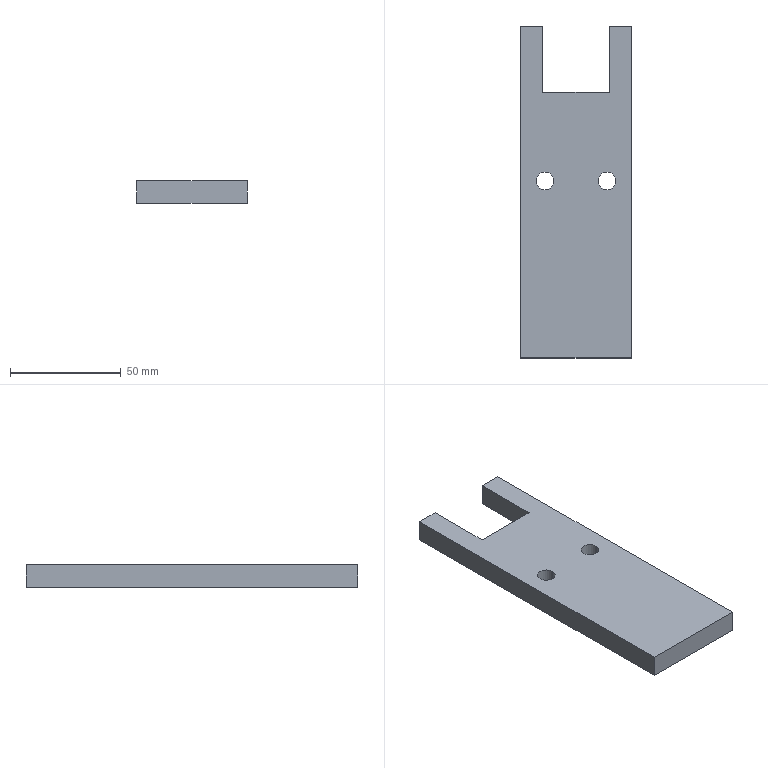Part | SolidWorks | features ICE 2, Extrusion 1 | 1 solid | 14 faces | box 50 x 150 x 10 mm | volume 64995 mm3 | plane 10 | cylinder 4 | commonest cylinder face diameters 8 x4
STEP:
#1=CARTESIAN_POINT('',(-18.,5.,0.));
#2=VERTEX_POINT('',#1);
#3=CARTESIAN_POINT('',(-10.,5.,0.));
#4=VERTEX_POINT('',#3);
#5=CARTESIAN_POINT('',(-14.,5.,0.));
#6=DIRECTION('',(0.,0.,1.));
#7=DIRECTION('',(1.,0.,0.));
#8=AXIS2_PLACEMENT_3D('',#5,#6,#7);
#9=CIRCLE('',#8,4.);
#10=EDGE_CURVE('',#2,#4,#9,.T.);
#11=ORIENTED_EDGE('',*,*,#10,.F.);
#12=CARTESIAN_POINT('',(-18.,5.,10.));
#13=VERTEX_POINT('',#12);
#14=CARTESIAN_POINT('',(-18.,5.,0.));
#15=DIRECTION('',(0.,0.,1.));
#16=VECTOR('',#15,1000.);
#17=LINE('',#14,#16);
#18=EDGE_CURVE('',#2,#13,#17,.T.);
#19=ORIENTED_EDGE('',*,*,#18,.T.);
#20=CARTESIAN_POINT('',(-10.,5.,10.));
#21=VERTEX_POINT('',#20);
#22=CARTESIAN_POINT('',(-14.,5.,10.));
#23=DIRECTION('',(0.,0.,1.));
#24=DIRECTION('',(1.,0.,0.));
#25=AXIS2_PLACEMENT_3D('',#22,#23,#24);
#26=CIRCLE('',#25,4.);
#27=EDGE_CURVE('',#13,#21,#26,.T.);
#28=ORIENTED_EDGE('',*,*,#27,.T.);
#29=CARTESIAN_POINT('',(-10.,5.,0.));
#30=DIRECTION('',(0.,0.,1.));
#31=VECTOR('',#30,1000.);
#32=LINE('',#29,#31);
#33=EDGE_CURVE('',#4,#21,#32,.T.);
#34=ORIENTED_EDGE('',*,*,#33,.F.);
#35=EDGE_LOOP('',(#11,#19,#28,#34));
#36=FACE_OUTER_BOUND('',#35,.T.);
#37=CARTESIAN_POINT('',(-14.,5.,0.));
#38=DIRECTION('',(0.,0.,1.));
#39=DIRECTION('',(1.,0.,0.));
#40=AXIS2_PLACEMENT_3D('',#37,#38,#39);
#41=CYLINDRICAL_SURFACE('',#40,4.);
#42=ADVANCED_FACE('',(#36),#41,.F.);
#43=CARTESIAN_POINT('',(10.,5.,0.));
#44=VERTEX_POINT('',#43);
#45=CARTESIAN_POINT('',(18.,5.,0.));
#46=VERTEX_POINT('',#45);
#47=CARTESIAN_POINT('',(14.,5.,0.));
#48=DIRECTION('',(0.,0.,1.));
#49=DIRECTION('',(-1.,0.,0.));
#50=AXIS2_PLACEMENT_3D('',#47,#48,#49);
#51=CIRCLE('',#50,4.);
#52=EDGE_CURVE('',#44,#46,#51,.T.);
#53=ORIENTED_EDGE('',*,*,#52,.F.);
#54=CARTESIAN_POINT('',(10.,5.,10.));
#55=VERTEX_POINT('',#54);
#56=CARTESIAN_POINT('',(10.,5.,0.));
#57=DIRECTION('',(0.,0.,1.));
#58=VECTOR('',#57,1000.);
#59=LINE('',#56,#58);
#60=EDGE_CURVE('',#44,#55,#59,.T.);
#61=ORIENTED_EDGE('',*,*,#60,.T.);
#62=CARTESIAN_POINT('',(18.,5.,10.));
#63=VERTEX_POINT('',#62);
#64=CARTESIAN_POINT('',(14.,5.,10.));
#65=DIRECTION('',(0.,0.,1.));
#66=DIRECTION('',(-1.,0.,0.));
#67=AXIS2_PLACEMENT_3D('',#64,#65,#66);
#68=CIRCLE('',#67,4.);
#69=EDGE_CURVE('',#55,#63,#68,.T.);
#70=ORIENTED_EDGE('',*,*,#69,.T.);
#71=CARTESIAN_POINT('',(18.,5.,0.));
#72=DIRECTION('',(0.,0.,1.));
#73=VECTOR('',#72,1000.);
#74=LINE('',#71,#73);
#75=EDGE_CURVE('',#46,#63,#74,.T.);
#76=ORIENTED_EDGE('',*,*,#75,.F.);
#77=EDGE_LOOP('',(#53,#61,#70,#76));
#78=FACE_OUTER_BOUND('',#77,.T.);
#79=CARTESIAN_POINT('',(14.,5.,0.));
#80=DIRECTION('',(0.,0.,1.));
#81=DIRECTION('',(1.,0.,0.));
#82=AXIS2_PLACEMENT_3D('',#79,#80,#81);
#83=CYLINDRICAL_SURFACE('',#82,4.);
#84=ADVANCED_FACE('',(#78),#83,.F.);
#85=CARTESIAN_POINT('',(-15.,75.,10.));
#86=VERTEX_POINT('',#85);
#87=CARTESIAN_POINT('',(-25.,75.,10.));
#88=VERTEX_POINT('',#87);
#89=CARTESIAN_POINT('',(-25.,75.,10.));
#90=DIRECTION('',(-1.,0.,0.));
#91=VECTOR('',#90,1000.);
#92=LINE('',#89,#91);
#93=EDGE_CURVE('',#86,#88,#92,.T.);
#94=ORIENTED_EDGE('',*,*,#93,.F.);
#95=CARTESIAN_POINT('',(-15.,75.,0.));
#96=VERTEX_POINT('',#95);
#97=CARTESIAN_POINT('',(-15.,75.,0.));
#98=DIRECTION('',(0.,0.,1.));
#99=VECTOR('',#98,1000.);
#100=LINE('',#97,#99);
#101=EDGE_CURVE('',#96,#86,#100,.T.);
#102=ORIENTED_EDGE('',*,*,#101,.F.);
#103=CARTESIAN_POINT('',(-25.,75.,0.));
#104=VERTEX_POINT('',#103);
#105=CARTESIAN_POINT('',(-25.,75.,0.));
#106=DIRECTION('',(-1.,0.,0.));
#107=VECTOR('',#106,1000.);
#108=LINE('',#105,#107);
#109=EDGE_CURVE('',#96,#104,#108,.T.);
#110=ORIENTED_EDGE('',*,*,#109,.T.);
#111=CARTESIAN_POINT('',(-25.,75.,10.));
#112=DIRECTION('',(0.,0.,-1.));
#113=VECTOR('',#112,1000.);
#114=LINE('',#111,#113);
#115=EDGE_CURVE('',#88,#104,#114,.T.);
#116=ORIENTED_EDGE('',*,*,#115,.F.);
#117=EDGE_LOOP('',(#94,#102,#110,#116));
#118=FACE_OUTER_BOUND('',#117,.T.);
#119=CARTESIAN_POINT('',(-25.,75.,10.));
#120=DIRECTION('',(0.,-1.,0.));
#121=DIRECTION('',(0.,0.,-1.));
#122=AXIS2_PLACEMENT_3D('',#119,#120,#121);
#123=PLANE('',#122);
#124=ADVANCED_FACE('',(#118),#123,.F.);
#125=CARTESIAN_POINT('',(25.,-75.,0.));
#126=VERTEX_POINT('',#125);
#127=CARTESIAN_POINT('',(25.,75.,0.));
#128=VERTEX_POINT('',#127);
#129=CARTESIAN_POINT('',(25.,-75.,0.));
#130=DIRECTION('',(0.,1.,0.));
#131=VECTOR('',#130,1000.);
#132=LINE('',#129,#131);
#133=EDGE_CURVE('',#126,#128,#132,.T.);
#134=ORIENTED_EDGE('',*,*,#133,.T.);
#135=CARTESIAN_POINT('',(25.,75.,10.));
#136=VERTEX_POINT('',#135);
#137=CARTESIAN_POINT('',(25.,75.,10.));
#138=DIRECTION('',(0.,0.,-1.));
#139=VECTOR('',#138,1000.);
#140=LINE('',#137,#139);
#141=EDGE_CURVE('',#136,#128,#140,.T.);
#142=ORIENTED_EDGE('',*,*,#141,.F.);
#143=CARTESIAN_POINT('',(25.,-75.,10.));
#144=VERTEX_POINT('',#143);
#145=CARTESIAN_POINT('',(25.,-75.,10.));
#146=DIRECTION('',(0.,1.,0.));
#147=VECTOR('',#146,1000.);
#148=LINE('',#145,#147);
#149=EDGE_CURVE('',#144,#136,#148,.T.);
#150=ORIENTED_EDGE('',*,*,#149,.F.);
#151=CARTESIAN_POINT('',(25.,-75.,10.));
#152=DIRECTION('',(0.,0.,-1.));
#153=VECTOR('',#152,1000.);
#154=LINE('',#151,#153);
#155=EDGE_CURVE('',#144,#126,#154,.T.);
#156=ORIENTED_EDGE('',*,*,#155,.T.);
#157=EDGE_LOOP('',(#134,#142,#150,#156));
#158=FACE_OUTER_BOUND('',#157,.T.);
#159=CARTESIAN_POINT('',(25.,-75.,10.));
#160=DIRECTION('',(-1.,0.,0.));
#161=DIRECTION('',(0.,0.,1.));
#162=AXIS2_PLACEMENT_3D('',#159,#160,#161);
#163=PLANE('',#162);
#164=ADVANCED_FACE('',(#158),#163,.F.);
#165=CARTESIAN_POINT('',(15.,75.,0.));
#166=VERTEX_POINT('',#165);
#167=CARTESIAN_POINT('',(-25.,75.,0.));
#168=DIRECTION('',(-1.,0.,0.));
#169=VECTOR('',#168,1000.);
#170=LINE('',#167,#169);
#171=EDGE_CURVE('',#128,#166,#170,.T.);
#172=ORIENTED_EDGE('',*,*,#171,.T.);
#173=CARTESIAN_POINT('',(15.,75.,10.));
#174=VERTEX_POINT('',#173);
#175=CARTESIAN_POINT('',(15.,75.,0.));
#176=DIRECTION('',(0.,0.,1.));
#177=VECTOR('',#176,1000.);
#178=LINE('',#175,#177);
#179=EDGE_CURVE('',#166,#174,#178,.T.);
#180=ORIENTED_EDGE('',*,*,#179,.T.);
#181=CARTESIAN_POINT('',(-25.,75.,10.));
#182=DIRECTION('',(-1.,0.,0.));
#183=VECTOR('',#182,1000.);
#184=LINE('',#181,#183);
#185=EDGE_CURVE('',#136,#174,#184,.T.);
#186=ORIENTED_EDGE('',*,*,#185,.F.);
#187=ORIENTED_EDGE('',*,*,#141,.T.);
#188=EDGE_LOOP('',(#172,#180,#186,#187));
#189=FACE_OUTER_BOUND('',#188,.T.);
#190=CARTESIAN_POINT('',(-25.,75.,10.));
#191=DIRECTION('',(0.,-1.,0.));
#192=DIRECTION('',(0.,0.,-1.));
#193=AXIS2_PLACEMENT_3D('',#190,#191,#192);
#194=PLANE('',#193);
#195=ADVANCED_FACE('',(#189),#194,.F.);
#196=CARTESIAN_POINT('',(-25.,-75.,0.));
#197=VERTEX_POINT('',#196);
#198=CARTESIAN_POINT('',(-25.,-75.,0.));
#199=DIRECTION('',(0.,-1.,0.));
#200=VECTOR('',#199,1000.);
#201=LINE('',#198,#200);
#202=EDGE_CURVE('',#104,#197,#201,.T.);
#203=ORIENTED_EDGE('',*,*,#202,.T.);
#204=CARTESIAN_POINT('',(-25.,-75.,10.));
#205=VERTEX_POINT('',#204);
#206=CARTESIAN_POINT('',(-25.,-75.,10.));
#207=DIRECTION('',(0.,0.,-1.));
#208=VECTOR('',#207,1000.);
#209=LINE('',#206,#208);
#210=EDGE_CURVE('',#205,#197,#209,.T.);
#211=ORIENTED_EDGE('',*,*,#210,.F.);
#212=CARTESIAN_POINT('',(-25.,-75.,10.));
#213=DIRECTION('',(0.,-1.,0.));
#214=VECTOR('',#213,1000.);
#215=LINE('',#212,#214);
#216=EDGE_CURVE('',#88,#205,#215,.T.);
#217=ORIENTED_EDGE('',*,*,#216,.F.);
#218=ORIENTED_EDGE('',*,*,#115,.T.);
#219=EDGE_LOOP('',(#203,#211,#217,#218));
#220=FACE_OUTER_BOUND('',#219,.T.);
#221=CARTESIAN_POINT('',(-25.,-75.,10.));
#222=DIRECTION('',(1.,0.,0.));
#223=DIRECTION('',(0.,0.,-1.));
#224=AXIS2_PLACEMENT_3D('',#221,#222,#223);
#225=PLANE('',#224);
#226=ADVANCED_FACE('',(#220),#225,.F.);
#227=CARTESIAN_POINT('',(-25.,-75.,0.));
#228=DIRECTION('',(1.,0.,0.));
#229=VECTOR('',#228,1000.);
#230=LINE('',#227,#229);
#231=EDGE_CURVE('',#197,#126,#230,.T.);
#232=ORIENTED_EDGE('',*,*,#231,.T.);
#233=ORIENTED_EDGE('',*,*,#155,.F.);
#234=CARTESIAN_POINT('',(-25.,-75.,10.));
#235=DIRECTION('',(1.,0.,0.));
#236=VECTOR('',#235,1000.);
#237=LINE('',#234,#236);
#238=EDGE_CURVE('',#205,#144,#237,.T.);
#239=ORIENTED_EDGE('',*,*,#238,.F.);
#240=ORIENTED_EDGE('',*,*,#210,.T.);
#241=EDGE_LOOP('',(#232,#233,#239,#240));
#242=FACE_OUTER_BOUND('',#241,.T.);
#243=CARTESIAN_POINT('',(-25.,-75.,10.));
#244=DIRECTION('',(0.,1.,0.));
#245=DIRECTION('',(0.,0.,1.));
#246=AXIS2_PLACEMENT_3D('',#243,#244,#245);
#247=PLANE('',#246);
#248=ADVANCED_FACE('',(#242),#247,.F.);
#249=CARTESIAN_POINT('',(-14.,5.,10.));
#250=DIRECTION('',(0.,0.,1.));
#251=DIRECTION('',(1.,0.,0.));
#252=AXIS2_PLACEMENT_3D('',#249,#250,#251);
#253=CIRCLE('',#252,4.);
#254=EDGE_CURVE('',#21,#13,#253,.T.);
#255=ORIENTED_EDGE('',*,*,#254,.F.);
#256=ORIENTED_EDGE('',*,*,#27,.F.);
#257=EDGE_LOOP('',(#255,#256));
#258=FACE_BOUND('',#257,.T.);
#259=CARTESIAN_POINT('',(14.,5.,10.));
#260=DIRECTION('',(0.,0.,1.));
#261=DIRECTION('',(-1.,0.,0.));
#262=AXIS2_PLACEMENT_3D('',#259,#260,#261);
#263=CIRCLE('',#262,4.);
#264=EDGE_CURVE('',#63,#55,#263,.T.);
#265=ORIENTED_EDGE('',*,*,#264,.F.);
#266=ORIENTED_EDGE('',*,*,#69,.F.);
#267=EDGE_LOOP('',(#265,#266));
#268=FACE_BOUND('',#267,.T.);
#269=CARTESIAN_POINT('',(-15.,45.,10.));
#270=VERTEX_POINT('',#269);
#271=CARTESIAN_POINT('',(15.,45.,10.));
#272=VERTEX_POINT('',#271);
#273=CARTESIAN_POINT('',(-15.,45.,10.));
#274=DIRECTION('',(1.,0.,0.));
#275=VECTOR('',#274,1000.);
#276=LINE('',#273,#275);
#277=EDGE_CURVE('',#270,#272,#276,.T.);
#278=ORIENTED_EDGE('',*,*,#277,.F.);
#279=CARTESIAN_POINT('',(-15.,75.,10.));
#280=DIRECTION('',(0.,-1.,0.));
#281=VECTOR('',#280,1000.);
#282=LINE('',#279,#281);
#283=EDGE_CURVE('',#86,#270,#282,.T.);
#284=ORIENTED_EDGE('',*,*,#283,.F.);
#285=ORIENTED_EDGE('',*,*,#93,.T.);
#286=ORIENTED_EDGE('',*,*,#216,.T.);
#287=ORIENTED_EDGE('',*,*,#238,.T.);
#288=ORIENTED_EDGE('',*,*,#149,.T.);
#289=ORIENTED_EDGE('',*,*,#185,.T.);
#290=CARTESIAN_POINT('',(15.,75.,10.));
#291=DIRECTION('',(0.,1.,0.));
#292=VECTOR('',#291,1000.);
#293=LINE('',#290,#292);
#294=EDGE_CURVE('',#272,#174,#293,.T.);
#295=ORIENTED_EDGE('',*,*,#294,.F.);
#296=EDGE_LOOP('',(#278,#284,#285,#286,#287,#288,#289,#295));
#297=FACE_OUTER_BOUND('',#296,.T.);
#298=CARTESIAN_POINT('',(0.,0.,10.));
#299=DIRECTION('',(0.,0.,-1.));
#300=DIRECTION('',(-1.,0.,0.));
#301=AXIS2_PLACEMENT_3D('',#298,#299,#300);
#302=PLANE('',#301);
#303=ADVANCED_FACE('',(#258,#268,#297),#302,.F.);
#304=CARTESIAN_POINT('',(-14.,5.,0.));
#305=DIRECTION('',(0.,0.,1.));
#306=DIRECTION('',(1.,0.,0.));
#307=AXIS2_PLACEMENT_3D('',#304,#305,#306);
#308=CIRCLE('',#307,4.);
#309=EDGE_CURVE('',#4,#2,#308,.T.);
#310=ORIENTED_EDGE('',*,*,#309,.T.);
#311=ORIENTED_EDGE('',*,*,#10,.T.);
#312=EDGE_LOOP('',(#310,#311));
#313=FACE_BOUND('',#312,.T.);
#314=CARTESIAN_POINT('',(14.,5.,0.));
#315=DIRECTION('',(0.,0.,1.));
#316=DIRECTION('',(-1.,0.,0.));
#317=AXIS2_PLACEMENT_3D('',#314,#315,#316);
#318=CIRCLE('',#317,4.);
#319=EDGE_CURVE('',#46,#44,#318,.T.);
#320=ORIENTED_EDGE('',*,*,#319,.T.);
#321=ORIENTED_EDGE('',*,*,#52,.T.);
#322=EDGE_LOOP('',(#320,#321));
#323=FACE_BOUND('',#322,.T.);
#324=CARTESIAN_POINT('',(-15.,45.,0.));
#325=VERTEX_POINT('',#324);
#326=CARTESIAN_POINT('',(-15.,75.,0.));
#327=DIRECTION('',(0.,-1.,0.));
#328=VECTOR('',#327,1000.);
#329=LINE('',#326,#328);
#330=EDGE_CURVE('',#96,#325,#329,.T.);
#331=ORIENTED_EDGE('',*,*,#330,.T.);
#332=CARTESIAN_POINT('',(15.,45.,0.));
#333=VERTEX_POINT('',#332);
#334=CARTESIAN_POINT('',(-15.,45.,0.));
#335=DIRECTION('',(1.,0.,0.));
#336=VECTOR('',#335,1000.);
#337=LINE('',#334,#336);
#338=EDGE_CURVE('',#325,#333,#337,.T.);
#339=ORIENTED_EDGE('',*,*,#338,.T.);
#340=CARTESIAN_POINT('',(15.,75.,0.));
#341=DIRECTION('',(0.,1.,0.));
#342=VECTOR('',#341,1000.);
#343=LINE('',#340,#342);
#344=EDGE_CURVE('',#333,#166,#343,.T.);
#345=ORIENTED_EDGE('',*,*,#344,.T.);
#346=ORIENTED_EDGE('',*,*,#171,.F.);
#347=ORIENTED_EDGE('',*,*,#133,.F.);
#348=ORIENTED_EDGE('',*,*,#231,.F.);
#349=ORIENTED_EDGE('',*,*,#202,.F.);
#350=ORIENTED_EDGE('',*,*,#109,.F.);
#351=EDGE_LOOP('',(#331,#339,#345,#346,#347,#348,#349,#350));
#352=FACE_OUTER_BOUND('',#351,.T.);
#353=CARTESIAN_POINT('',(0.,0.,0.));
#354=DIRECTION('',(0.,0.,-1.));
#355=DIRECTION('',(-1.,0.,0.));
#356=AXIS2_PLACEMENT_3D('',#353,#354,#355);
#357=PLANE('',#356);
#358=ADVANCED_FACE('',(#313,#323,#352),#357,.T.);
#359=ORIENTED_EDGE('',*,*,#283,.T.);
#360=CARTESIAN_POINT('',(-15.,45.,0.));
#361=DIRECTION('',(0.,0.,1.));
#362=VECTOR('',#361,1000.);
#363=LINE('',#360,#362);
#364=EDGE_CURVE('',#325,#270,#363,.T.);
#365=ORIENTED_EDGE('',*,*,#364,.F.);
#366=ORIENTED_EDGE('',*,*,#330,.F.);
#367=ORIENTED_EDGE('',*,*,#101,.T.);
#368=EDGE_LOOP('',(#359,#365,#366,#367));
#369=FACE_OUTER_BOUND('',#368,.T.);
#370=CARTESIAN_POINT('',(-15.,75.,0.));
#371=DIRECTION('',(-1.,0.,0.));
#372=DIRECTION('',(0.,-1.,0.));
#373=AXIS2_PLACEMENT_3D('',#370,#371,#372);
#374=PLANE('',#373);
#375=ADVANCED_FACE('',(#369),#374,.F.);
#376=ORIENTED_EDGE('',*,*,#294,.T.);
#377=ORIENTED_EDGE('',*,*,#179,.F.);
#378=ORIENTED_EDGE('',*,*,#344,.F.);
#379=CARTESIAN_POINT('',(15.,45.,0.));
#380=DIRECTION('',(0.,0.,1.));
#381=VECTOR('',#380,1000.);
#382=LINE('',#379,#381);
#383=EDGE_CURVE('',#333,#272,#382,.T.);
#384=ORIENTED_EDGE('',*,*,#383,.T.);
#385=EDGE_LOOP('',(#376,#377,#378,#384));
#386=FACE_OUTER_BOUND('',#385,.T.);
#387=CARTESIAN_POINT('',(15.,75.,0.));
#388=DIRECTION('',(1.,0.,0.));
#389=DIRECTION('',(0.,1.,0.));
#390=AXIS2_PLACEMENT_3D('',#387,#388,#389);
#391=PLANE('',#390);
#392=ADVANCED_FACE('',(#386),#391,.F.);
#393=ORIENTED_EDGE('',*,*,#277,.T.);
#394=ORIENTED_EDGE('',*,*,#383,.F.);
#395=ORIENTED_EDGE('',*,*,#338,.F.);
#396=ORIENTED_EDGE('',*,*,#364,.T.);
#397=EDGE_LOOP('',(#393,#394,#395,#396));
#398=FACE_OUTER_BOUND('',#397,.T.);
#399=CARTESIAN_POINT('',(-15.,45.,0.));
#400=DIRECTION('',(0.,-1.,0.));
#401=DIRECTION('',(0.,0.,-1.));
#402=AXIS2_PLACEMENT_3D('',#399,#400,#401);
#403=PLANE('',#402);
#404=ADVANCED_FACE('',(#398),#403,.F.);
#405=ORIENTED_EDGE('',*,*,#60,.F.);
#406=ORIENTED_EDGE('',*,*,#319,.F.);
#407=ORIENTED_EDGE('',*,*,#75,.T.);
#408=ORIENTED_EDGE('',*,*,#264,.T.);
#409=EDGE_LOOP('',(#405,#406,#407,#408));
#410=FACE_OUTER_BOUND('',#409,.T.);
#411=CARTESIAN_POINT('',(14.,5.,0.));
#412=DIRECTION('',(0.,0.,1.));
#413=DIRECTION('',(1.,0.,0.));
#414=AXIS2_PLACEMENT_3D('',#411,#412,#413);
#415=CYLINDRICAL_SURFACE('',#414,4.);
#416=ADVANCED_FACE('',(#410),#415,.F.);
#417=ORIENTED_EDGE('',*,*,#18,.F.);
#418=ORIENTED_EDGE('',*,*,#309,.F.);
#419=ORIENTED_EDGE('',*,*,#33,.T.);
#420=ORIENTED_EDGE('',*,*,#254,.T.);
#421=EDGE_LOOP('',(#417,#418,#419,#420));
#422=FACE_OUTER_BOUND('',#421,.T.);
#423=CARTESIAN_POINT('',(-14.,5.,0.));
#424=DIRECTION('',(0.,0.,1.));
#425=DIRECTION('',(1.,0.,0.));
#426=AXIS2_PLACEMENT_3D('',#423,#424,#425);
#427=CYLINDRICAL_SURFACE('',#426,4.);
#428=ADVANCED_FACE('',(#422),#427,.F.);
#429=CLOSED_SHELL('',(#42,#84,#124,#164,#195,#226,#248,#303,#358,#375,#392,#404,#416,#428));
#430=MANIFOLD_SOLID_BREP('',#429);
#431=CARTESIAN_POINT('',(0.,0.,0.));
#432=DIRECTION('',(0.,0.,1.));
#433=DIRECTION('',(1.,0.,0.));
#434=AXIS2_PLACEMENT_3D('',#431,#432,#433);
#435=(LENGTH_UNIT()NAMED_UNIT(*)SI_UNIT(.MILLI.,.METRE.));
#436=UNCERTAINTY_MEASURE_WITH_UNIT(LENGTH_MEASURE(0.00001),#435,'','');
#437=(NAMED_UNIT(*)PLANE_ANGLE_UNIT()SI_UNIT($,.RADIAN.));
#438=(NAMED_UNIT(*)SI_UNIT($,.STERADIAN.)SOLID_ANGLE_UNIT());
#439=(GEOMETRIC_REPRESENTATION_CONTEXT(3)GLOBAL_UNCERTAINTY_ASSIGNED_CONTEXT((#436))GLOBAL_UNIT_ASSIGNED_CONTEXT((#435,#437,#438))REPRESENTATION_CONTEXT('',''));
#440=ADVANCED_BREP_SHAPE_REPRESENTATION('',(#430,#434),#439);